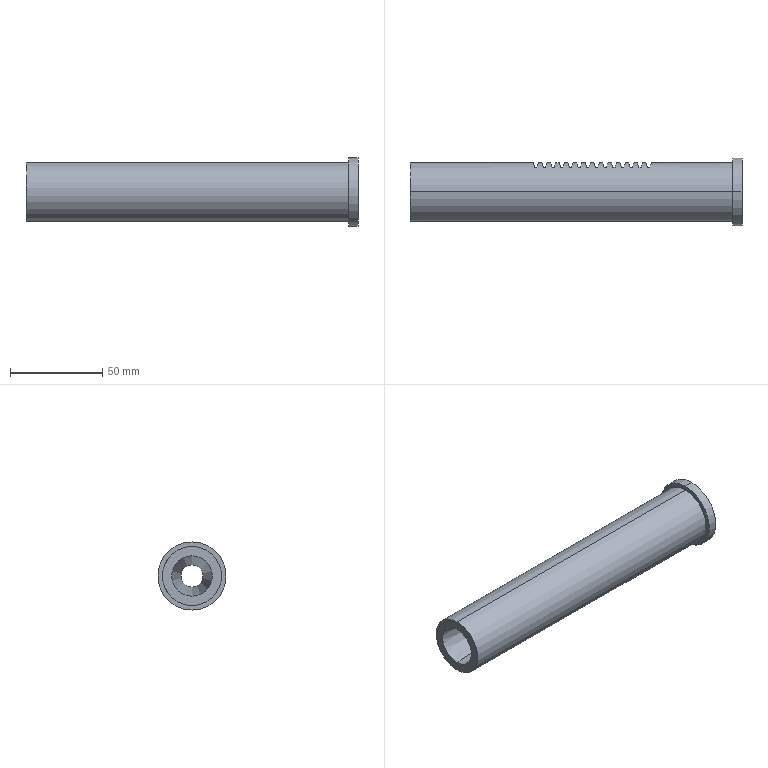Part | SolidWorks | features ICE 4, Extrusion 1, RevCut 1 | 1 solid | 56 faces | box 180 x 37 x 37 mm | volume 98767 mm3 | plane 46 | cylinder 8 | cone 2 | commonest cylinder face diameters 12 x2 20 x2 32 x2 37 x2